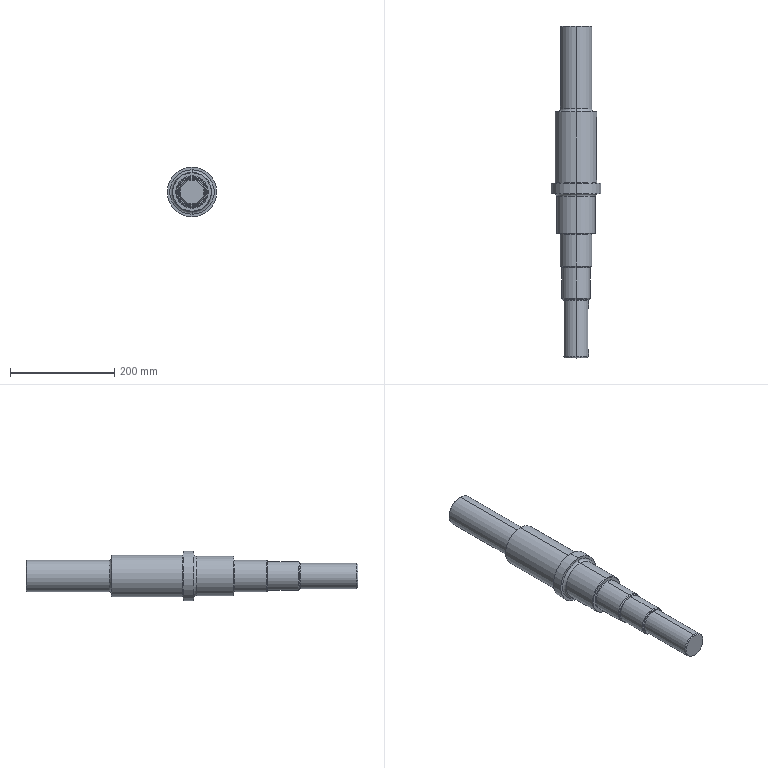Part | SolidWorks | features Chamfer 4, Fillet 3, ICE 2, HoleWzd 1, Revolution 1 | 1 solid | 64 faces | box 95 x 636 x 95 mm | volume 2135437 mm3 | cylinder 22 | cone 16 | plane 14 | torus 12 | commonest cylinder face diameters 8.5 x4 60 x4 14 x2 22 x2 48 x2 55 x2